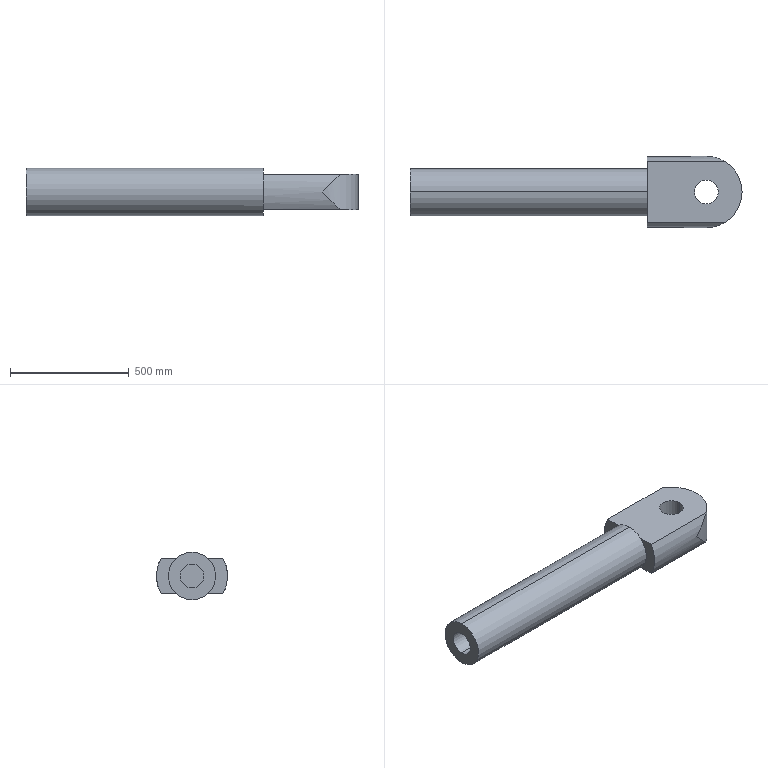Part | SolidWorks | features ICE 3, Extrusion 1 | 1 solid | 18 faces | box 1400 x 300 x 200 mm | volume 38372929 mm3 | cylinder 10 | plane 8 | commonest cylinder face diameters 100 x4 300 x4 200 x2
STEP:
#1=CARTESIAN_POINT('',(1200.,0.,-75.));
#2=VERTEX_POINT('',#1);
#3=CARTESIAN_POINT('',(1300.,0.,-75.));
#4=VERTEX_POINT('',#3);
#5=CARTESIAN_POINT('',(1250.,0.,-75.));
#6=DIRECTION('',(0.,0.,1.));
#7=DIRECTION('',(1.,0.,0.));
#8=AXIS2_PLACEMENT_3D('',#5,#6,#7);
#9=CIRCLE('',#8,50.);
#10=EDGE_CURVE('',#2,#4,#9,.T.);
#11=ORIENTED_EDGE('',*,*,#10,.F.);
#12=CARTESIAN_POINT('',(1200.,0.,75.));
#13=VERTEX_POINT('',#12);
#14=CARTESIAN_POINT('',(1200.,0.,-100.));
#15=DIRECTION('',(0.,0.,1.));
#16=VECTOR('',#15,1000.);
#17=LINE('',#14,#16);
#18=EDGE_CURVE('',#2,#13,#17,.T.);
#19=ORIENTED_EDGE('',*,*,#18,.T.);
#20=CARTESIAN_POINT('',(1300.,0.,75.));
#21=VERTEX_POINT('',#20);
#22=CARTESIAN_POINT('',(1250.,0.,75.));
#23=DIRECTION('',(0.,0.,-1.));
#24=DIRECTION('',(0.,1.,0.));
#25=AXIS2_PLACEMENT_3D('',#22,#23,#24);
#26=CIRCLE('',#25,50.);
#27=EDGE_CURVE('',#21,#13,#26,.T.);
#28=ORIENTED_EDGE('',*,*,#27,.F.);
#29=CARTESIAN_POINT('',(1300.,0.,-100.));
#30=DIRECTION('',(0.,0.,1.));
#31=VECTOR('',#30,1000.);
#32=LINE('',#29,#31);
#33=EDGE_CURVE('',#4,#21,#32,.T.);
#34=ORIENTED_EDGE('',*,*,#33,.F.);
#35=EDGE_LOOP('',(#11,#19,#28,#34));
#36=FACE_OUTER_BOUND('',#35,.T.);
#37=CARTESIAN_POINT('',(1250.,0.,-100.));
#38=DIRECTION('',(0.,0.,1.));
#39=DIRECTION('',(1.,0.,0.));
#40=AXIS2_PLACEMENT_3D('',#37,#38,#39);
#41=CYLINDRICAL_SURFACE('',#40,50.);
#42=ADVANCED_FACE('',(#36),#41,.F.);
#43=CARTESIAN_POINT('',(1325.,-129.904,-75.));
#44=VERTEX_POINT('',#43);
#45=CARTESIAN_POINT('',(1400.,0.,-75.));
#46=VERTEX_POINT('',#45);
#47=CARTESIAN_POINT('',(1250.,0.,-75.));
#48=DIRECTION('',(0.,0.,1.));
#49=DIRECTION('',(1.,0.,0.));
#50=AXIS2_PLACEMENT_3D('',#47,#48,#49);
#51=CIRCLE('',#50,150.);
#52=EDGE_CURVE('',#44,#46,#51,.T.);
#53=ORIENTED_EDGE('',*,*,#52,.T.);
#54=CARTESIAN_POINT('',(1400.,0.,75.));
#55=VERTEX_POINT('',#54);
#56=CARTESIAN_POINT('',(1400.,0.,-100.));
#57=DIRECTION('',(0.,0.,1.));
#58=VECTOR('',#57,1000.);
#59=LINE('',#56,#58);
#60=EDGE_CURVE('',#46,#55,#59,.T.);
#61=ORIENTED_EDGE('',*,*,#60,.T.);
#62=CARTESIAN_POINT('',(1325.,-129.904,75.));
#63=VERTEX_POINT('',#62);
#64=CARTESIAN_POINT('',(1250.,0.,75.));
#65=DIRECTION('',(0.,0.,-1.));
#66=DIRECTION('',(0.,1.,0.));
#67=AXIS2_PLACEMENT_3D('',#64,#65,#66);
#68=CIRCLE('',#67,150.);
#69=EDGE_CURVE('',#55,#63,#68,.T.);
#70=ORIENTED_EDGE('',*,*,#69,.T.);
#71=CARTESIAN_POINT('',(1250.,-150.,0.));
#72=VERTEX_POINT('',#71);
#73=CARTESIAN_POINT('',(1325.,-129.904,75.));
#74=CARTESIAN_POINT('',(1302.065,-143.146,52.065));
#75=CARTESIAN_POINT('',(1276.484,-150.,26.484));
#76=CARTESIAN_POINT('',(1250.,-150.,0.));
#77=(BOUNDED_CURVE()B_SPLINE_CURVE(3,(#73,#74,#75,#76),.UNSPECIFIED.,.F.,.T.)B_SPLINE_CURVE_WITH_KNOTS((4,4),(4.189,4.712),.UNSPECIFIED.)CURVE()GEOMETRIC_REPRESENTATION_ITEM()RATIONAL_B_SPLINE_CURVE((1.,0.9773,0.9773,1.))REPRESENTATION_ITEM(''));
#78=EDGE_CURVE('',#63,#72,#77,.T.);
#79=ORIENTED_EDGE('',*,*,#78,.T.);
#80=CARTESIAN_POINT('',(1250.,-150.,0.));
#81=CARTESIAN_POINT('',(1276.484,-150.,-26.484));
#82=CARTESIAN_POINT('',(1302.065,-143.146,-52.065));
#83=CARTESIAN_POINT('',(1325.,-129.904,-75.));
#84=(BOUNDED_CURVE()B_SPLINE_CURVE(3,(#80,#81,#82,#83),.UNSPECIFIED.,.F.,.T.)B_SPLINE_CURVE_WITH_KNOTS((4,4),(1.571,2.094),.UNSPECIFIED.)CURVE()GEOMETRIC_REPRESENTATION_ITEM()RATIONAL_B_SPLINE_CURVE((1.,0.9773,0.9773,1.))REPRESENTATION_ITEM(''));
#85=EDGE_CURVE('',#72,#44,#84,.T.);
#86=ORIENTED_EDGE('',*,*,#85,.T.);
#87=EDGE_LOOP('',(#53,#61,#70,#79,#86));
#88=FACE_OUTER_BOUND('',#87,.T.);
#89=CARTESIAN_POINT('',(1250.,0.,-100.));
#90=DIRECTION('',(0.,0.,1.));
#91=DIRECTION('',(1.,0.,0.));
#92=AXIS2_PLACEMENT_3D('',#89,#90,#91);
#93=CYLINDRICAL_SURFACE('',#92,150.);
#94=ADVANCED_FACE('',(#88),#93,.T.);
#95=CARTESIAN_POINT('',(1000.,0.,50.));
#96=VERTEX_POINT('',#95);
#97=CARTESIAN_POINT('',(1000.,0.,-50.));
#98=VERTEX_POINT('',#97);
#99=CARTESIAN_POINT('',(1000.,0.,0.));
#100=DIRECTION('',(1.,0.,0.));
#101=DIRECTION('',(0.,0.,-1.));
#102=AXIS2_PLACEMENT_3D('',#99,#100,#101);
#103=CIRCLE('',#102,50.);
#104=EDGE_CURVE('',#96,#98,#103,.T.);
#105=ORIENTED_EDGE('',*,*,#104,.T.);
#106=CARTESIAN_POINT('',(0.,0.,-50.));
#107=VERTEX_POINT('',#106);
#108=CARTESIAN_POINT('',(1000.,0.,-50.));
#109=DIRECTION('',(-1.,0.,0.));
#110=VECTOR('',#109,1000.);
#111=LINE('',#108,#110);
#112=EDGE_CURVE('',#98,#107,#111,.T.);
#113=ORIENTED_EDGE('',*,*,#112,.T.);
#114=CARTESIAN_POINT('',(0.,0.,50.));
#115=VERTEX_POINT('',#114);
#116=CARTESIAN_POINT('',(0.,0.,0.));
#117=DIRECTION('',(1.,0.,0.));
#118=DIRECTION('',(0.,0.,-1.));
#119=AXIS2_PLACEMENT_3D('',#116,#117,#118);
#120=CIRCLE('',#119,50.);
#121=EDGE_CURVE('',#115,#107,#120,.T.);
#122=ORIENTED_EDGE('',*,*,#121,.F.);
#123=CARTESIAN_POINT('',(1000.,0.,50.));
#124=DIRECTION('',(-1.,0.,0.));
#125=VECTOR('',#124,1000.);
#126=LINE('',#123,#125);
#127=EDGE_CURVE('',#96,#115,#126,.T.);
#128=ORIENTED_EDGE('',*,*,#127,.F.);
#129=EDGE_LOOP('',(#105,#113,#122,#128));
#130=FACE_OUTER_BOUND('',#129,.T.);
#131=CARTESIAN_POINT('',(1000.,0.,0.));
#132=DIRECTION('',(-1.,0.,0.));
#133=DIRECTION('',(0.,0.,1.));
#134=AXIS2_PLACEMENT_3D('',#131,#132,#133);
#135=CYLINDRICAL_SURFACE('',#134,50.);
#136=ADVANCED_FACE('',(#130),#135,.F.);
#137=CARTESIAN_POINT('',(1000.,0.,-100.));
#138=VERTEX_POINT('',#137);
#139=CARTESIAN_POINT('',(1000.,66.144,-75.));
#140=VERTEX_POINT('',#139);
#141=CARTESIAN_POINT('',(1000.,0.,0.));
#142=DIRECTION('',(1.,0.,0.));
#143=DIRECTION('',(0.,0.,-1.));
#144=AXIS2_PLACEMENT_3D('',#141,#142,#143);
#145=CIRCLE('',#144,100.);
#146=EDGE_CURVE('',#138,#140,#145,.T.);
#147=ORIENTED_EDGE('',*,*,#146,.F.);
#148=CARTESIAN_POINT('',(0.,0.,-100.));
#149=VERTEX_POINT('',#148);
#150=CARTESIAN_POINT('',(1000.,0.,-100.));
#151=DIRECTION('',(-1.,0.,0.));
#152=VECTOR('',#151,1000.);
#153=LINE('',#150,#152);
#154=EDGE_CURVE('',#138,#149,#153,.T.);
#155=ORIENTED_EDGE('',*,*,#154,.T.);
#156=CARTESIAN_POINT('',(0.,0.,100.));
#157=VERTEX_POINT('',#156);
#158=CARTESIAN_POINT('',(0.,0.,0.));
#159=DIRECTION('',(1.,0.,0.));
#160=DIRECTION('',(0.,0.,-1.));
#161=AXIS2_PLACEMENT_3D('',#158,#159,#160);
#162=CIRCLE('',#161,100.);
#163=EDGE_CURVE('',#149,#157,#162,.T.);
#164=ORIENTED_EDGE('',*,*,#163,.T.);
#165=CARTESIAN_POINT('',(1000.,0.,100.));
#166=VERTEX_POINT('',#165);
#167=CARTESIAN_POINT('',(1000.,0.,100.));
#168=DIRECTION('',(-1.,0.,0.));
#169=VECTOR('',#168,1000.);
#170=LINE('',#167,#169);
#171=EDGE_CURVE('',#166,#157,#170,.T.);
#172=ORIENTED_EDGE('',*,*,#171,.F.);
#173=CARTESIAN_POINT('',(1000.,66.144,75.));
#174=VERTEX_POINT('',#173);
#175=CARTESIAN_POINT('',(1000.,0.,0.));
#176=DIRECTION('',(1.,0.,0.));
#177=DIRECTION('',(0.,0.,-1.));
#178=AXIS2_PLACEMENT_3D('',#175,#176,#177);
#179=CIRCLE('',#178,100.);
#180=EDGE_CURVE('',#174,#166,#179,.T.);
#181=ORIENTED_EDGE('',*,*,#180,.F.);
#182=CARTESIAN_POINT('',(1000.,0.,0.));
#183=DIRECTION('',(1.,0.,0.));
#184=DIRECTION('',(0.,0.,-1.));
#185=AXIS2_PLACEMENT_3D('',#182,#183,#184);
#186=CIRCLE('',#185,100.);
#187=EDGE_CURVE('',#140,#174,#186,.T.);
#188=ORIENTED_EDGE('',*,*,#187,.F.);
#189=EDGE_LOOP('',(#147,#155,#164,#172,#181,#188));
#190=FACE_OUTER_BOUND('',#189,.T.);
#191=CARTESIAN_POINT('',(1000.,0.,0.));
#192=DIRECTION('',(-1.,0.,0.));
#193=DIRECTION('',(0.,0.,1.));
#194=AXIS2_PLACEMENT_3D('',#191,#192,#193);
#195=CYLINDRICAL_SURFACE('',#194,100.);
#196=ADVANCED_FACE('',(#190),#195,.T.);
#197=ORIENTED_EDGE('',*,*,#27,.T.);
#198=CARTESIAN_POINT('',(1250.,0.,75.));
#199=DIRECTION('',(0.,0.,-1.));
#200=DIRECTION('',(0.,1.,0.));
#201=AXIS2_PLACEMENT_3D('',#198,#199,#200);
#202=CIRCLE('',#201,50.);
#203=EDGE_CURVE('',#13,#21,#202,.T.);
#204=ORIENTED_EDGE('',*,*,#203,.T.);
#205=EDGE_LOOP('',(#197,#204));
#206=FACE_BOUND('',#205,.T.);
#207=CARTESIAN_POINT('',(1325.,129.904,75.));
#208=VERTEX_POINT('',#207);
#209=CARTESIAN_POINT('',(1250.,0.,75.));
#210=DIRECTION('',(0.,0.,-1.));
#211=DIRECTION('',(0.,1.,0.));
#212=AXIS2_PLACEMENT_3D('',#209,#210,#211);
#213=CIRCLE('',#212,150.);
#214=EDGE_CURVE('',#208,#55,#213,.T.);
#215=ORIENTED_EDGE('',*,*,#214,.F.);
#216=CARTESIAN_POINT('',(1000.,129.904,75.));
#217=VERTEX_POINT('',#216);
#218=CARTESIAN_POINT('',(1400.,129.904,75.));
#219=DIRECTION('',(-1.,0.,0.));
#220=VECTOR('',#219,1000.);
#221=LINE('',#218,#220);
#222=EDGE_CURVE('',#208,#217,#221,.T.);
#223=ORIENTED_EDGE('',*,*,#222,.T.);
#224=CARTESIAN_POINT('',(1000.,129.904,75.));
#225=DIRECTION('',(0.,-1.,0.));
#226=VECTOR('',#225,1000.);
#227=LINE('',#224,#226);
#228=EDGE_CURVE('',#217,#174,#227,.T.);
#229=ORIENTED_EDGE('',*,*,#228,.T.);
#230=CARTESIAN_POINT('',(1000.,-66.144,75.));
#231=VERTEX_POINT('',#230);
#232=CARTESIAN_POINT('',(1000.,129.904,75.));
#233=DIRECTION('',(0.,-1.,0.));
#234=VECTOR('',#233,1000.);
#235=LINE('',#232,#234);
#236=EDGE_CURVE('',#174,#231,#235,.T.);
#237=ORIENTED_EDGE('',*,*,#236,.T.);
#238=CARTESIAN_POINT('',(1000.,-129.904,75.));
#239=VERTEX_POINT('',#238);
#240=CARTESIAN_POINT('',(1000.,129.904,75.));
#241=DIRECTION('',(0.,-1.,0.));
#242=VECTOR('',#241,1000.);
#243=LINE('',#240,#242);
#244=EDGE_CURVE('',#231,#239,#243,.T.);
#245=ORIENTED_EDGE('',*,*,#244,.T.);
#246=CARTESIAN_POINT('',(1400.,-129.904,75.));
#247=DIRECTION('',(-1.,0.,0.));
#248=VECTOR('',#247,1000.);
#249=LINE('',#246,#248);
#250=EDGE_CURVE('',#63,#239,#249,.T.);
#251=ORIENTED_EDGE('',*,*,#250,.F.);
#252=ORIENTED_EDGE('',*,*,#69,.F.);
#253=EDGE_LOOP('',(#215,#223,#229,#237,#245,#251,#252));
#254=FACE_OUTER_BOUND('',#253,.T.);
#255=CARTESIAN_POINT('',(1400.,129.904,75.));
#256=DIRECTION('',(0.,0.,-1.));
#257=DIRECTION('',(0.,1.,0.));
#258=AXIS2_PLACEMENT_3D('',#255,#256,#257);
#259=PLANE('',#258);
#260=ADVANCED_FACE('',(#206,#254),#259,.F.);
#261=CARTESIAN_POINT('',(1250.,150.,0.));
#262=VERTEX_POINT('',#261);
#263=CARTESIAN_POINT('',(1250.,150.,0.));
#264=CARTESIAN_POINT('',(1276.484,150.,26.484));
#265=CARTESIAN_POINT('',(1302.065,143.146,52.065));
#266=CARTESIAN_POINT('',(1325.,129.904,75.));
#267=(BOUNDED_CURVE()B_SPLINE_CURVE(3,(#263,#264,#265,#266),.UNSPECIFIED.,.F.,.F.)B_SPLINE_CURVE_WITH_KNOTS((4,4),(1.571,2.094),.UNSPECIFIED.)CURVE()GEOMETRIC_REPRESENTATION_ITEM()RATIONAL_B_SPLINE_CURVE((1.,0.9773,0.9773,1.))REPRESENTATION_ITEM(''));
#268=EDGE_CURVE('',#262,#208,#267,.T.);
#269=ORIENTED_EDGE('',*,*,#268,.F.);
#270=CARTESIAN_POINT('',(1325.,129.904,-75.));
#271=VERTEX_POINT('',#270);
#272=CARTESIAN_POINT('',(1325.,129.904,-75.));
#273=CARTESIAN_POINT('',(1302.065,143.146,-52.065));
#274=CARTESIAN_POINT('',(1276.484,150.,-26.484));
#275=CARTESIAN_POINT('',(1250.,150.,0.));
#276=(BOUNDED_CURVE()B_SPLINE_CURVE(3,(#272,#273,#274,#275),.UNSPECIFIED.,.F.,.F.)B_SPLINE_CURVE_WITH_KNOTS((4,4),(4.189,4.712),.UNSPECIFIED.)CURVE()GEOMETRIC_REPRESENTATION_ITEM()RATIONAL_B_SPLINE_CURVE((1.,0.9773,0.9773,1.))REPRESENTATION_ITEM(''));
#277=EDGE_CURVE('',#271,#262,#276,.T.);
#278=ORIENTED_EDGE('',*,*,#277,.F.);
#279=CARTESIAN_POINT('',(1000.,129.904,-75.));
#280=VERTEX_POINT('',#279);
#281=CARTESIAN_POINT('',(1400.,129.904,-75.));
#282=DIRECTION('',(-1.,0.,0.));
#283=VECTOR('',#282,1000.);
#284=LINE('',#281,#283);
#285=EDGE_CURVE('',#271,#280,#284,.T.);
#286=ORIENTED_EDGE('',*,*,#285,.T.);
#287=CARTESIAN_POINT('',(1000.,0.,0.));
#288=DIRECTION('',(1.,0.,0.));
#289=DIRECTION('',(0.,0.,-1.));
#290=AXIS2_PLACEMENT_3D('',#287,#288,#289);
#291=CIRCLE('',#290,150.);
#292=EDGE_CURVE('',#280,#217,#291,.T.);
#293=ORIENTED_EDGE('',*,*,#292,.T.);
#294=ORIENTED_EDGE('',*,*,#222,.F.);
#295=EDGE_LOOP('',(#269,#278,#286,#293,#294));
#296=FACE_OUTER_BOUND('',#295,.T.);
#297=CARTESIAN_POINT('',(1400.,0.,0.));
#298=DIRECTION('',(-1.,0.,0.));
#299=DIRECTION('',(0.,0.,1.));
#300=AXIS2_PLACEMENT_3D('',#297,#298,#299);
#301=CYLINDRICAL_SURFACE('',#300,150.);
#302=ADVANCED_FACE('',(#296),#301,.T.);
#303=CARTESIAN_POINT('',(1250.,0.,-75.));
#304=DIRECTION('',(0.,0.,1.));
#305=DIRECTION('',(1.,0.,0.));
#306=AXIS2_PLACEMENT_3D('',#303,#304,#305);
#307=CIRCLE('',#306,50.);
#308=EDGE_CURVE('',#4,#2,#307,.T.);
#309=ORIENTED_EDGE('',*,*,#308,.T.);
#310=ORIENTED_EDGE('',*,*,#10,.T.);
#311=EDGE_LOOP('',(#309,#310));
#312=FACE_BOUND('',#311,.T.);
#313=ORIENTED_EDGE('',*,*,#52,.F.);
#314=CARTESIAN_POINT('',(1000.,-129.904,-75.));
#315=VERTEX_POINT('',#314);
#316=CARTESIAN_POINT('',(1400.,-129.904,-75.));
#317=DIRECTION('',(-1.,0.,0.));
#318=VECTOR('',#317,1000.);
#319=LINE('',#316,#318);
#320=EDGE_CURVE('',#44,#315,#319,.T.);
#321=ORIENTED_EDGE('',*,*,#320,.T.);
#322=CARTESIAN_POINT('',(1000.,-66.144,-75.));
#323=VERTEX_POINT('',#322);
#324=CARTESIAN_POINT('',(1000.,129.904,-75.));
#325=DIRECTION('',(0.,1.,0.));
#326=VECTOR('',#325,1000.);
#327=LINE('',#324,#326);
#328=EDGE_CURVE('',#315,#323,#327,.T.);
#329=ORIENTED_EDGE('',*,*,#328,.T.);
#330=CARTESIAN_POINT('',(1000.,129.904,-75.));
#331=DIRECTION('',(0.,1.,0.));
#332=VECTOR('',#331,1000.);
#333=LINE('',#330,#332);
#334=EDGE_CURVE('',#323,#140,#333,.T.);
#335=ORIENTED_EDGE('',*,*,#334,.T.);
#336=CARTESIAN_POINT('',(1000.,129.904,-75.));
#337=DIRECTION('',(0.,1.,0.));
#338=VECTOR('',#337,1000.);
#339=LINE('',#336,#338);
#340=EDGE_CURVE('',#140,#280,#339,.T.);
#341=ORIENTED_EDGE('',*,*,#340,.T.);
#342=ORIENTED_EDGE('',*,*,#285,.F.);
#343=CARTESIAN_POINT('',(1250.,0.,-75.));
#344=DIRECTION('',(0.,0.,1.));
#345=DIRECTION('',(1.,0.,0.));
#346=AXIS2_PLACEMENT_3D('',#343,#344,#345);
#347=CIRCLE('',#346,150.);
#348=EDGE_CURVE('',#46,#271,#347,.T.);
#349=ORIENTED_EDGE('',*,*,#348,.F.);
#350=EDGE_LOOP('',(#313,#321,#329,#335,#341,#342,#349));
#351=FACE_OUTER_BOUND('',#350,.T.);
#352=CARTESIAN_POINT('',(1400.,129.904,-75.));
#353=DIRECTION('',(0.,0.,1.));
#354=DIRECTION('',(1.,0.,0.));
#355=AXIS2_PLACEMENT_3D('',#352,#353,#354);
#356=PLANE('',#355);
#357=ADVANCED_FACE('',(#312,#351),#356,.F.);
#358=ORIENTED_EDGE('',*,*,#78,.F.);
#359=ORIENTED_EDGE('',*,*,#250,.T.);
#360=CARTESIAN_POINT('',(1000.,0.,0.));
#361=DIRECTION('',(1.,0.,0.));
#362=DIRECTION('',(0.,0.,-1.));
#363=AXIS2_PLACEMENT_3D('',#360,#361,#362);
#364=CIRCLE('',#363,150.);
#365=EDGE_CURVE('',#239,#315,#364,.T.);
#366=ORIENTED_EDGE('',*,*,#365,.T.);
#367=ORIENTED_EDGE('',*,*,#320,.F.);
#368=ORIENTED_EDGE('',*,*,#85,.F.);
#369=EDGE_LOOP('',(#358,#359,#366,#367,#368));
#370=FACE_OUTER_BOUND('',#369,.T.);
#371=CARTESIAN_POINT('',(1400.,0.,0.));
#372=DIRECTION('',(-1.,0.,0.));
#373=DIRECTION('',(0.,0.,1.));
#374=AXIS2_PLACEMENT_3D('',#371,#372,#373);
#375=CYLINDRICAL_SURFACE('',#374,150.);
#376=ADVANCED_FACE('',(#370),#375,.T.);
#377=ORIENTED_EDGE('',*,*,#236,.F.);
#378=ORIENTED_EDGE('',*,*,#180,.T.);
#379=CARTESIAN_POINT('',(1000.,0.,0.));
#380=DIRECTION('',(1.,0.,0.));
#381=DIRECTION('',(0.,0.,-1.));
#382=AXIS2_PLACEMENT_3D('',#379,#380,#381);
#383=CIRCLE('',#382,100.);
#384=EDGE_CURVE('',#166,#231,#383,.T.);
#385=ORIENTED_EDGE('',*,*,#384,.T.);
#386=EDGE_LOOP('',(#377,#378,#385));
#387=FACE_OUTER_BOUND('',#386,.T.);
#388=CARTESIAN_POINT('',(1000.,0.,0.));
#389=DIRECTION('',(1.,0.,0.));
#390=DIRECTION('',(0.,0.,-1.));
#391=AXIS2_PLACEMENT_3D('',#388,#389,#390);
#392=PLANE('',#391);
#393=ADVANCED_FACE('',(#387),#392,.T.);
#394=ORIENTED_EDGE('',*,*,#334,.F.);
#395=CARTESIAN_POINT('',(1000.,0.,0.));
#396=DIRECTION('',(1.,0.,0.));
#397=DIRECTION('',(0.,0.,-1.));
#398=AXIS2_PLACEMENT_3D('',#395,#396,#397);
#399=CIRCLE('',#398,100.);
#400=EDGE_CURVE('',#323,#138,#399,.T.);
#401=ORIENTED_EDGE('',*,*,#400,.T.);
#402=ORIENTED_EDGE('',*,*,#146,.T.);
#403=EDGE_LOOP('',(#394,#401,#402));
#404=FACE_OUTER_BOUND('',#403,.T.);
#405=CARTESIAN_POINT('',(1000.,0.,0.));
#406=DIRECTION('',(1.,0.,0.));
#407=DIRECTION('',(0.,0.,-1.));
#408=AXIS2_PLACEMENT_3D('',#405,#406,#407);
#409=PLANE('',#408);
#410=ADVANCED_FACE('',(#404),#409,.T.);
#411=CARTESIAN_POINT('',(0.,0.,0.));
#412=DIRECTION('',(1.,0.,0.));
#413=DIRECTION('',(0.,0.,-1.));
#414=AXIS2_PLACEMENT_3D('',#411,#412,#413);
#415=CIRCLE('',#414,100.);
#416=EDGE_CURVE('',#157,#149,#415,.T.);
#417=ORIENTED_EDGE('',*,*,#416,.F.);
#418=ORIENTED_EDGE('',*,*,#163,.F.);
#419=EDGE_LOOP('',(#417,#418));
#420=FACE_OUTER_BOUND('',#419,.T.);
#421=ORIENTED_EDGE('',*,*,#121,.T.);
#422=CARTESIAN_POINT('',(0.,0.,0.));
#423=DIRECTION('',(1.,0.,0.));
#424=DIRECTION('',(0.,0.,-1.));
#425=AXIS2_PLACEMENT_3D('',#422,#423,#424);
#426=CIRCLE('',#425,50.);
#427=EDGE_CURVE('',#107,#115,#426,.T.);
#428=ORIENTED_EDGE('',*,*,#427,.T.);
#429=EDGE_LOOP('',(#421,#428));
#430=FACE_BOUND('',#429,.T.);
#431=CARTESIAN_POINT('',(0.,0.,0.));
#432=DIRECTION('',(1.,0.,0.));
#433=DIRECTION('',(0.,0.,-1.));
#434=AXIS2_PLACEMENT_3D('',#431,#432,#433);
#435=PLANE('',#434);
#436=ADVANCED_FACE('',(#420,#430),#435,.F.);
#437=ORIENTED_EDGE('',*,*,#154,.F.);
#438=ORIENTED_EDGE('',*,*,#400,.F.);
#439=CARTESIAN_POINT('',(1000.,0.,0.));
#440=DIRECTION('',(1.,0.,0.));
#441=DIRECTION('',(0.,0.,-1.));
#442=AXIS2_PLACEMENT_3D('',#439,#440,#441);
#443=CIRCLE('',#442,100.);
#444=EDGE_CURVE('',#231,#323,#443,.T.);
#445=ORIENTED_EDGE('',*,*,#444,.F.);
#446=ORIENTED_EDGE('',*,*,#384,.F.);
#447=ORIENTED_EDGE('',*,*,#171,.T.);
#448=ORIENTED_EDGE('',*,*,#416,.T.);
#449=EDGE_LOOP('',(#437,#438,#445,#446,#447,#448));
#450=FACE_OUTER_BOUND('',#449,.T.);
#451=CARTESIAN_POINT('',(1000.,0.,0.));
#452=DIRECTION('',(-1.,0.,0.));
#453=DIRECTION('',(0.,0.,1.));
#454=AXIS2_PLACEMENT_3D('',#451,#452,#453);
#455=CYLINDRICAL_SURFACE('',#454,100.);
#456=ADVANCED_FACE('',(#450),#455,.T.);
#457=ORIENTED_EDGE('',*,*,#112,.F.);
#458=CARTESIAN_POINT('',(1000.,0.,0.));
#459=DIRECTION('',(1.,0.,0.));
#460=DIRECTION('',(0.,0.,-1.));
#461=AXIS2_PLACEMENT_3D('',#458,#459,#460);
#462=CIRCLE('',#461,50.);
#463=EDGE_CURVE('',#98,#96,#462,.T.);
#464=ORIENTED_EDGE('',*,*,#463,.T.);
#465=ORIENTED_EDGE('',*,*,#127,.T.);
#466=ORIENTED_EDGE('',*,*,#427,.F.);
#467=EDGE_LOOP('',(#457,#464,#465,#466));
#468=FACE_OUTER_BOUND('',#467,.T.);
#469=CARTESIAN_POINT('',(1000.,0.,0.));
#470=DIRECTION('',(-1.,0.,0.));
#471=DIRECTION('',(0.,0.,1.));
#472=AXIS2_PLACEMENT_3D('',#469,#470,#471);
#473=CYLINDRICAL_SURFACE('',#472,50.);
#474=ADVANCED_FACE('',(#468),#473,.F.);
#475=ORIENTED_EDGE('',*,*,#244,.F.);
#476=ORIENTED_EDGE('',*,*,#444,.T.);
#477=ORIENTED_EDGE('',*,*,#328,.F.);
#478=ORIENTED_EDGE('',*,*,#365,.F.);
#479=EDGE_LOOP('',(#475,#476,#477,#478));
#480=FACE_OUTER_BOUND('',#479,.T.);
#481=CARTESIAN_POINT('',(1000.,0.,0.));
#482=DIRECTION('',(1.,0.,0.));
#483=DIRECTION('',(0.,0.,-1.));
#484=AXIS2_PLACEMENT_3D('',#481,#482,#483);
#485=PLANE('',#484);
#486=ADVANCED_FACE('',(#480),#485,.F.);
#487=ORIENTED_EDGE('',*,*,#340,.F.);
#488=ORIENTED_EDGE('',*,*,#187,.T.);
#489=ORIENTED_EDGE('',*,*,#228,.F.);
#490=ORIENTED_EDGE('',*,*,#292,.F.);
#491=EDGE_LOOP('',(#487,#488,#489,#490));
#492=FACE_OUTER_BOUND('',#491,.T.);
#493=CARTESIAN_POINT('',(1000.,0.,0.));
#494=DIRECTION('',(1.,0.,0.));
#495=DIRECTION('',(0.,0.,-1.));
#496=AXIS2_PLACEMENT_3D('',#493,#494,#495);
#497=PLANE('',#496);
#498=ADVANCED_FACE('',(#492),#497,.F.);
#499=ORIENTED_EDGE('',*,*,#104,.F.);
#500=ORIENTED_EDGE('',*,*,#463,.F.);
#501=EDGE_LOOP('',(#499,#500));
#502=FACE_OUTER_BOUND('',#501,.T.);
#503=CARTESIAN_POINT('',(1000.,0.,0.));
#504=DIRECTION('',(1.,0.,0.));
#505=DIRECTION('',(0.,0.,-1.));
#506=AXIS2_PLACEMENT_3D('',#503,#504,#505);
#507=PLANE('',#506);
#508=ADVANCED_FACE('',(#502),#507,.F.);
#509=ORIENTED_EDGE('',*,*,#60,.F.);
#510=ORIENTED_EDGE('',*,*,#348,.T.);
#511=ORIENTED_EDGE('',*,*,#277,.T.);
#512=ORIENTED_EDGE('',*,*,#268,.T.);
#513=ORIENTED_EDGE('',*,*,#214,.T.);
#514=EDGE_LOOP('',(#509,#510,#511,#512,#513));
#515=FACE_OUTER_BOUND('',#514,.T.);
#516=CARTESIAN_POINT('',(1250.,0.,-100.));
#517=DIRECTION('',(0.,0.,1.));
#518=DIRECTION('',(1.,0.,0.));
#519=AXIS2_PLACEMENT_3D('',#516,#517,#518);
#520=CYLINDRICAL_SURFACE('',#519,150.);
#521=ADVANCED_FACE('',(#515),#520,.T.);
#522=ORIENTED_EDGE('',*,*,#18,.F.);
#523=ORIENTED_EDGE('',*,*,#308,.F.);
#524=ORIENTED_EDGE('',*,*,#33,.T.);
#525=ORIENTED_EDGE('',*,*,#203,.F.);
#526=EDGE_LOOP('',(#522,#523,#524,#525));
#527=FACE_OUTER_BOUND('',#526,.T.);
#528=CARTESIAN_POINT('',(1250.,0.,-100.));
#529=DIRECTION('',(0.,0.,1.));
#530=DIRECTION('',(1.,0.,0.));
#531=AXIS2_PLACEMENT_3D('',#528,#529,#530);
#532=CYLINDRICAL_SURFACE('',#531,50.);
#533=ADVANCED_FACE('',(#527),#532,.F.);
#534=CLOSED_SHELL('',(#42,#94,#136,#196,#260,#302,#357,#376,#393,#410,#436,#456,#474,#486,#498,#508,#521,#533));
#535=MANIFOLD_SOLID_BREP('',#534);
#536=CARTESIAN_POINT('',(0.,0.,0.));
#537=DIRECTION('',(0.,0.,1.));
#538=DIRECTION('',(1.,0.,0.));
#539=AXIS2_PLACEMENT_3D('',#536,#537,#538);
#540=(LENGTH_UNIT()NAMED_UNIT(*)SI_UNIT(.MILLI.,.METRE.));
#541=UNCERTAINTY_MEASURE_WITH_UNIT(LENGTH_MEASURE(0.00001),#540,'','');
#542=(NAMED_UNIT(*)PLANE_ANGLE_UNIT()SI_UNIT($,.RADIAN.));
#543=(NAMED_UNIT(*)SI_UNIT($,.STERADIAN.)SOLID_ANGLE_UNIT());
#544=(GEOMETRIC_REPRESENTATION_CONTEXT(3)GLOBAL_UNCERTAINTY_ASSIGNED_CONTEXT((#541))GLOBAL_UNIT_ASSIGNED_CONTEXT((#540,#542,#543))REPRESENTATION_CONTEXT('',''));
#545=ADVANCED_BREP_SHAPE_REPRESENTATION('',(#535,#539),#544);